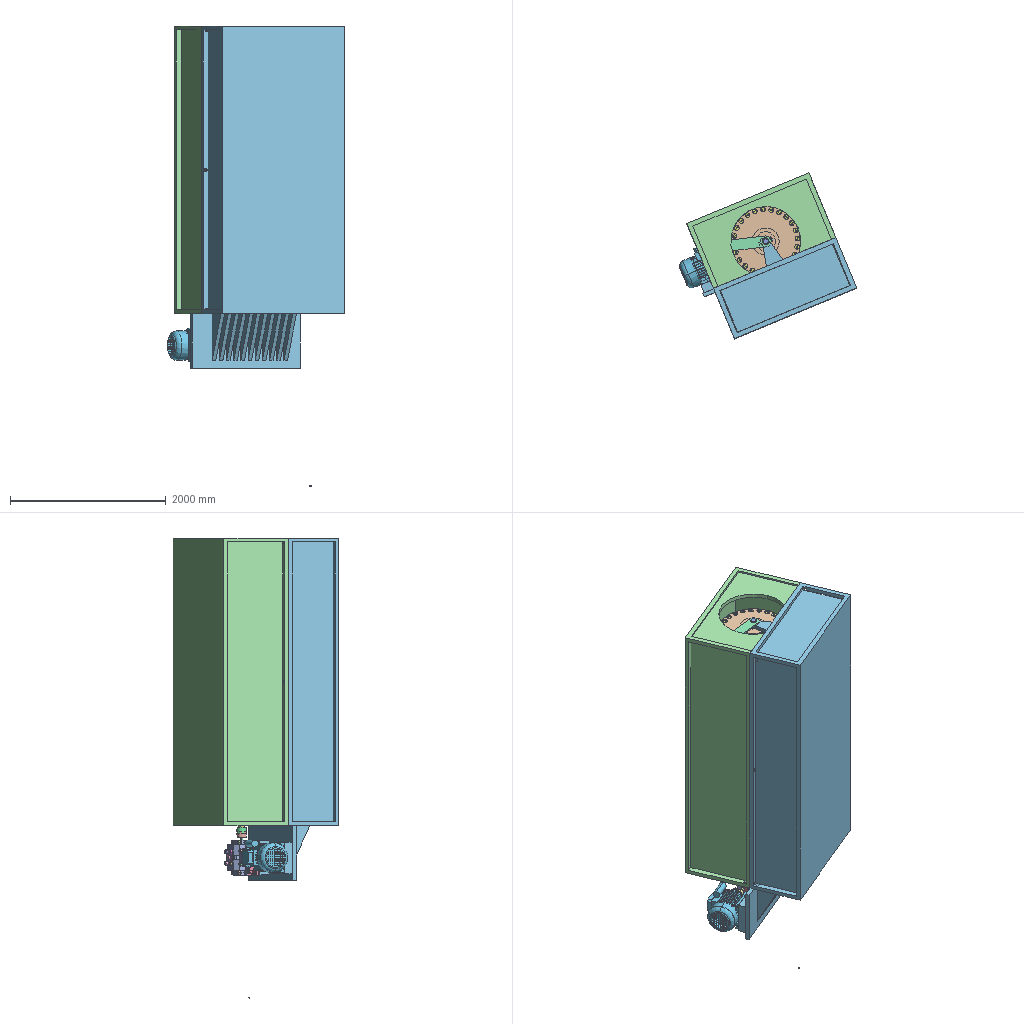Assembly | SolidWorks | 46 different items | 737 placed | box 2279 x 2129 x 5915 mm
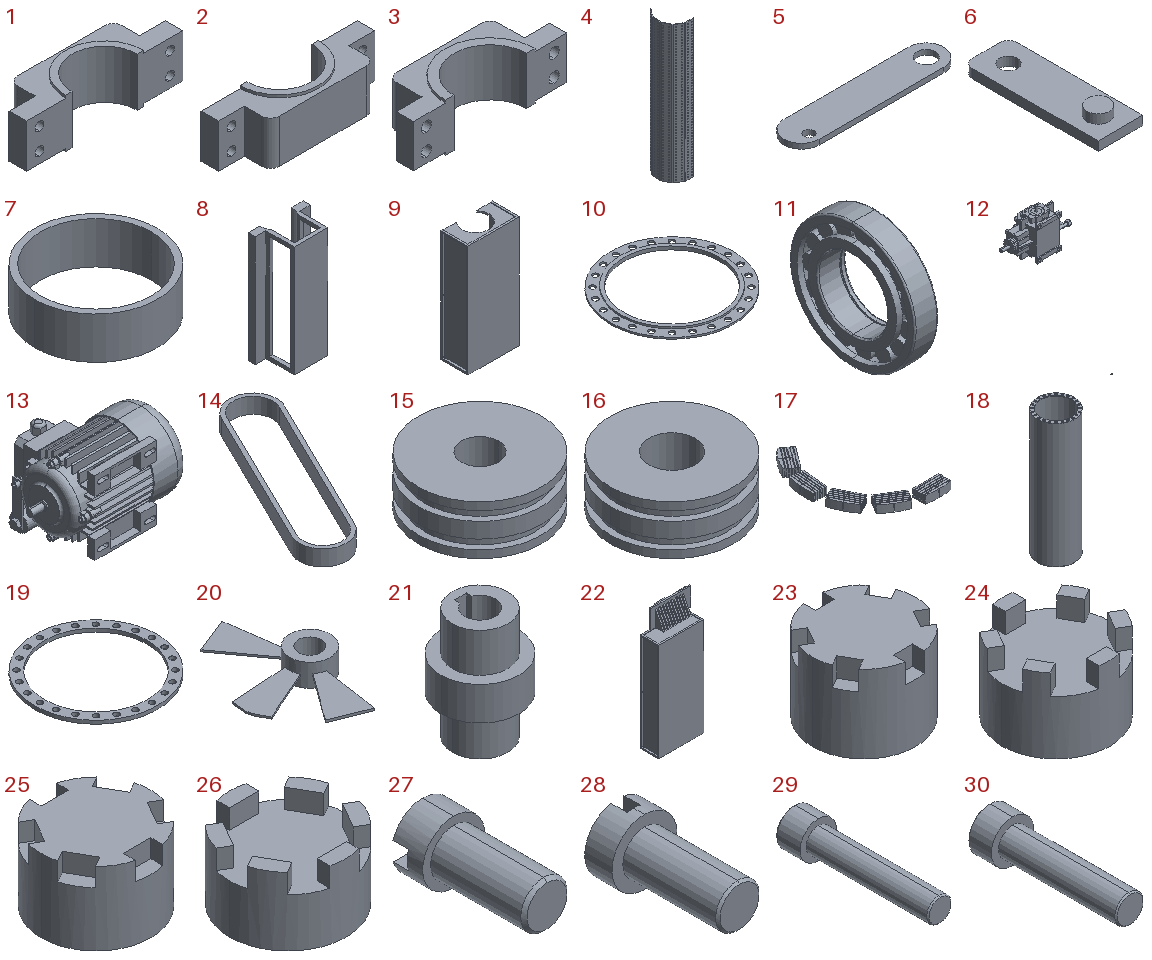Parts list (item | name | quantity | size | volume | features):
1 | - | x1 | 180 x 50 x 56 mm | 246956 mm3 | features ICE 4, Extrusion 1, Fillet 1, MirrorPattern 1
2 | - | x1 | 180 x 50 x 56 mm | 246956 mm3 | features ICE 4, Extrusion 1, Fillet 1, MirrorPattern 1
3 | - | x1 | 180 x 60 x 56 mm | 275897 mm3 | features ICE 4, Extrusion 1, Fillet 1, MirrorPattern 1
4 | - | x1 | 439.055 x 638.053 x 2960 mm | 32951018 mm3 | features ICE 7, 3DProfileFeature 3, Extrusion 1
5 | - | x1 | 640 x 140 x 20 mm | 1594386 mm3 | features Extrusion 1
6 | - | x1 | 100 x 300 x 40 mm | 610704 mm3 | features Extrusion 1, Fillet 1, ICE 1
7 | - | x1 | 100 x 100 x 34 mm | 50737 mm3 | features Extrusion 1
8 | - | x1 | 1550 x 1000 x 3127 mm | 797777759 mm3 | features ICE 10, Extrusion 1, MirrorPattern 1
9 | - | x1 | 1700 x 900 x 3700 mm | 580031915 mm3 | features ICE 37, Extrusion 1
10 | - | x1 | 900 x 900 x 25 mm | 3394255 mm3 | features ICE 3, Extrusion 1
11 | - | x2 | 40.8 x 180 x 180 mm | 440374 mm3 | features Revolution 4, CirPattern 1
12 | - | x1 | 1119 x 581.368 x 2095 mm | 29257315 mm3 | features BaseBody 37, Scale 1
13 | - | x1 | 643.342 x 464.31 x 414 mm | 44090407 mm3 | features ICE 21, Fillet 3, CirPattern 2, Revolution 2, LPattern 1, Scale 1
14 | - | x1 | 578.858 x 932.782 x 80 mm | 3573726 mm3 | features Extrusion 1
15 | - | x1 | 200 x 200 x 80 mm | 2108009 mm3 | features Extrusion 1, ICE 1, MirrorPattern 1
16 | - | x1 | 200 x 200 x 80 mm | 1980774 mm3 | features Extrusion 1, ICE 1, MirrorPattern 1
17 | - | x56 | 525 x 761.019 x 50 mm | 2587889 mm3 | features ICE 9, Extrusion 1
18 | - | x1 | 900 x 900 x 3000 mm | 71509466 mm3 | features ICE 2, Extrusion 1, MirrorPattern 1
19 | - | x1 | 900 x 900 x 25 mm | 4105669 mm3 | features ICE 2, Extrusion 1
20 | - | x17 | 431.967 x 677.234 x 100 mm | 2444150 mm3 | features ICE 4, Extrusion 1
21 | - | x1 | 70 x 70 x 100 mm | 224245 mm3 | features ICE 5, Extrusion 1
22 | - | x1 | 1850 x 1000 x 4400 mm | 1049313623 mm3 | features ICE 35, LPattern 2, Extrusion 1
23 | - | x1 | 80 x 80 x 60 mm | 237992 mm3 | features ICE 3, Extrusion 1
24 | - | x1 | 80 x 80 x 55 mm | 187551 mm3 | features ICE 3, Extrusion 1
25 | - | x1 | 120 x 120 x 80 mm | 586209 mm3 | features ICE 3, Extrusion 1
26 | - | x1 | 120 x 120 x 70 mm | 595667 mm3 | features ICE 3, Extrusion 1
27 | - | x560 | 20 x 40 x 20 mm | 7759 mm3 | features ICE 2, Chamfer 1, Extrusion 1
28 | - | x48 | 60 x 112.5 x 60 mm | 169671 mm3 | features ICE 2, Chamfer 1, Extrusion 1
29 | - | x4 | 15 x 60 x 15 mm | 5685 mm3 | features Chamfer 1, Extrusion 1, ICE 1
30 | - | x4 | 18 x 60 x 18 mm | 8188 mm3 | features Chamfer 1, Extrusion 1, ICE 1
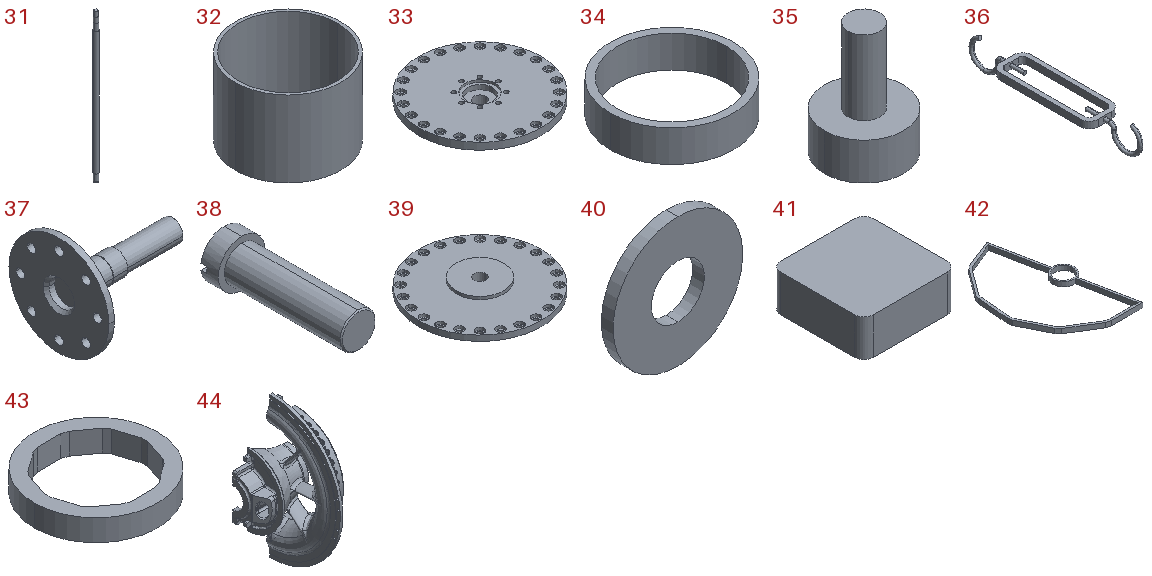31 | - | x1 | 100 x 100 x 3375 mm | 25329647 mm3 | features ICE 7, Chamfer 1, Extrusion 1
32 | - | x1 | 90 x 90 x 65 mm | 44670 mm3 | features Extrusion 1
33 | - | x1 | 900 x 900 x 130 mm | 35744082 mm3 | features ICE 6, CirPattern 2, Fillet 2, Extrusion 1, HoleWzd 1
34 | - | x1 | 85 x 85 x 22 mm | 27646 mm3 | features Extrusion 1
35 | - | x1 | 149.5 x 149.5 x 210 mm | 1568199 mm3 | features ICE 2, Extrusion 1
36 | - | x1 | 70 x 388 x 65.733 mm | 95929 mm3 | features Extrusion 1, ICE 1, MirrorPattern 1, Sweep 1
37 | - | x1 | 400 x 350 x 350 mm | 4309933 mm3 | features ICE 3, Chamfer 2, Revolution 1
38 | - | x8 | 40 x 115 x 40 mm | 88492 mm3 | features ICE 2, Chamfer 1, Extrusion 1
39 | - | x1 | 900 x 900 x 90 mm | 25700427 mm3 | features ICE 3, CirPattern 1, Extrusion 1, HoleWzd 1
40 | - | x1 | 220 x 20 x 220 mm | 633031 mm3 | features Extrusion 1
41 | - | x1 | 100 x 100 x 40 mm | 264030 mm3 | features Extrusion 1, Fillet 1, ICE 1
42 | - | x1 | 439.055 x 701.743 x 25 mm | 573866 mm3 | features ICE 2, Extrusion 1
43 | - | x1 | 884 x 884 x 155 mm | 38209027 mm3 | features Extrusion 1
44 | - | x1 | 985 x 1100 x 2200 mm | 275101534 mm3 | features MBimport 1
45 | UnnamedUnit | x1 | - | - | -
46 | Unnamed UnnamedGearUnnamedUnit (subassembly) | x1 | - | - | -
Mates (type | each side: item.copy, entity, surface, feature):
Concentric | 18.1 face cylinder Boss-Extrude 1 | 31.1 face cylinder Boss-Extrude 4
Concentric | 33.1 face cylinder Cut-Extrude 2 | 11.1 face cylinder Base-Revolve
Coincident | 11.1 face plane Boss-Revolve 2 | 40.1 face plane Boss-Extrude 1
Concentric | 18.1 face cylinder Cut-Extrude 1 | 33.1 face cylinder CirPattern 1
Concentric | 11.1 face cylinder Base-Revolve | 7.1 face cylinder Boss-Extrude 1
Coincident | 11.1 face plane Boss-Revolve 3 | 7.1 face plane Boss-Extrude 1
Concentric | 31.1 face cylinder Boss-Extrude 3 | 19.1 face cylinder Cut-Extrude 2
Concentric | 18.1 face cylinder Cut-Extrude 1 | 19.1 face cylinder Cut-Extrude 1
Coincident | 18.1 face plane Boss-Extrude 1 | 19.1 face plane Boss-Extrude 1
Coincident | 33.1 face plane Boss-Extrude 1 | 19.1 face plane Boss-Extrude 1
Concentric | 31.1 face cylinder Boss-Extrude 5 | 10.1 face cylinder Cut-Extrude 3
Concentric | 18.1 face cylinder Cut-Extrude 1 | 10.1 face cylinder Cut-Extrude 2
Coincident | 18.1 face plane Boss-Extrude 1 | 10.1 face plane Boss-Extrude 1
Concentric | 31.1 face cylinder Boss-Extrude 6 | 32.1 face cylinder Boss-Extrude 1
Concentric | 31.1 face cylinder Boss-Extrude 7 | 39.1 face cylinder Boss-Extrude 1
Concentric | 10.1 face cylinder Cut-Extrude 2 | 39.1 face cylinder CirPattern 1
Coincident | 10.1 face plane Boss-Extrude 1 | 39.1 face plane Boss-Extrude 1
Concentric | 31.1 face cylinder Boss-Extrude 7 | 34.1 face cylinder Boss-Extrude 1
Coincident | 39.1 face plane Boss-Extrude 3 | 34.1 edge
Coincident | 18.1 face plane Boss-Extrude 1 | 31.1 face plane Boss-Extrude 4
Concentric | 39.1 face cylinder Cut-Extrude 1 | 11.2 face cylinder Base-Revolve
Coincident | 39.1 face plane Boss-Extrude 1 | 11.2 face plane Boss-Revolve 2
Coincident | 31.1 face plane Boss-Extrude 5 | 32.1 face plane Boss-Extrude 1
Concentric | 31.1 face cylinder Boss-Extrude 7 | 2.1 face cylinder Cut-Extrude 1
Coincident | 39.1 face plane Boss-Extrude 3 | 2.1 face plane Mirror 1
Coincident | 10.1 face plane Boss-Extrude 2 | 4.1 face plane Boss-Extrude 1
Concentric | 18.1 face cylinder Boss-Extrude 1 | 17.1 face cylinder Boss-Extrude 1
Concentric | 39.1 face cylinder CirPattern 1 | 28.1 face cylinder Boss-Extrude 1
Coincident | 39.1 edge | 28.1 edge
Concentric | 33.1 face cylinder CirPattern 1 | 28.2 face cylinder Boss-Extrude 1
Coincident | 33.1 edge | 28.2 face plane Boss-Extrude 2
Concentric | 31.1 face cylinder Boss-Extrude 4 | 20.1 face cylinder Boss-Extrude 3
DistanceDim | 20.1 face plane Boss-Extrude 2 | 33.1 face plane Boss-Extrude 1
Coincident | 22.1 face plane | 5.1 face plane Boss-Extrude 1
Concentric | 22.1 edge | 6.1 edge
Coincident | 22.1 face plane | 6.1 face plane Boss-Extrude 2
Parallel | 36.1 edge | assembly select_type:10
Parallel | 3.1 edge | 22.1 face plane
Concentric | 2.1 face cylinder Cut-Extrude 2 | 29.1 face cylinder Boss-Extrude 1
Coincident | 2.1 face plane Boss-Extrude 3 | 29.1 face plane Boss-Extrude 2
Concentric | 2.1 face cylinder Cut-Extrude 2 | 29.2 face cylinder Boss-Extrude 1
Coincident | 2.1 face plane Boss-Extrude 3 | 29.2 face plane Boss-Extrude 2
Concentric | 2.1 face cylinder Cut-Extrude 2 | 29.3 face cylinder Boss-Extrude 1
Coincident | 2.1 face plane Boss-Extrude 3 | 29.3 edge
Concentric | 2.1 face cylinder Cut-Extrude 2 | 29.4 face cylinder Boss-Extrude 1
Coincident | 2.1 face plane Boss-Extrude 3 | 29.4 face plane Boss-Extrude 2
Concentric | 3.1 face cylinder Cut-Extrude 2 | 30.1 face cylinder Boss-Extrude 1
Coincident | 3.1 face plane Boss-Extrude 2 | 30.1 face plane Boss-Extrude 2
Concentric | 3.1 face cylinder Cut-Extrude 2 | 30.2 face cylinder Boss-Extrude 1
Coincident | 3.1 face plane Boss-Extrude 2 | 30.2 face plane Boss-Extrude 2
Concentric | 3.1 face cylinder Cut-Extrude 2 | 30.3 face cylinder Boss-Extrude 1
Coincident | 3.1 face plane Boss-Extrude 2 | 30.3 edge
Concentric | 3.1 edge | 30.4 face cylinder Boss-Extrude 1
Coincident | 3.1 face plane Boss-Extrude 2 | 30.4 face plane Boss-Extrude 2
Concentric | 17.1 face cylinder Cut-Extrude 9 | 4.1 face cylinder Cut-Extrude 5
Concentric | 4.1 edge | 27.1 face cylinder Boss-Extrude 1
Coincident | 4.1 face plane Boss-Extrude 1 | 27.1 edge
Concentric | 4.1 face cylinder Cut-Extrude 5 | 27.2 face cylinder Boss-Extrude 1
Coincident | 4.1 face plane Boss-Extrude 1 | 27.2 edge
Concentric | 4.1 face cylinder Cut-Extrude 6 | 27.3 face cylinder Boss-Extrude 1
Coincident | 4.1 face plane Boss-Extrude 1 | 27.3 face plane Boss-Extrude 2
Concentric | 4.1 face cylinder Cut-Extrude 6 | 27.4 face cylinder Boss-Extrude 1
Coincident | 4.1 face plane Boss-Extrude 1 | 27.4 edge
Concentric | 4.1 face cylinder Cut-Extrude 3 | 27.5 face cylinder Boss-Extrude 1
Coincident | 4.1 face plane Boss-Extrude 1 | 27.5 edge
Concentric | 4.1 edge | 27.6 face cylinder Boss-Extrude 1
Coincident | 4.1 face plane Boss-Extrude 1 | 27.6 face plane Boss-Extrude 2
Concentric | 4.1 edge | 27.7 face cylinder Boss-Extrude 1
Coincident | 4.1 face plane Boss-Extrude 1 | 27.7 edge
Concentric | 4.1 face cylinder Cut-Extrude 2 | 27.8 face cylinder Boss-Extrude 1
Coincident | 4.1 face plane Boss-Extrude 1 | 27.8 edge
Concentric | 4.1 edge | 27.9 face cylinder Boss-Extrude 1
Coincident | 4.1 face plane Boss-Extrude 1 | 27.9 edge
Concentric | 4.1 face cylinder Cut-Extrude 1 | 27.10 face cylinder Boss-Extrude 1
Coincident | 4.1 face plane Boss-Extrude 1 | 27.10 face plane Boss-Extrude 2
Coincident | 4.1 edge | 20.1 face plane Boss-Extrude 1
Coincident | 4.1 edge | 17.2 face plane Cut-Extrude 2
Parallel | 27.1 edge | 4.1 edge
Concentric | 31.1 face cylinder Boss-Extrude 3 | 22.1 face cylinder
Concentric | 22.1 edge | 29.3 face cylinder Boss-Extrude 1
Concentric | 22.1 face cylinder | 30.1 face cylinder Boss-Extrude 1
Coincident | 3.1 face plane Boss-Extrude 1 | 22.1 face plane
Concentric | 33.1 edge | 37.1 face cylinder Cut-Extrude 3
Concentric | 37.1 face cylinder Cut-Extrude 3 | 38.1 face cylinder Boss-Extrude 1
Concentric | 31.1 face cylinder Boss-Extrude 3 | 40.1 face cylinder Boss-Extrude 1
Coincident | 33.1 face plane Boss-Extrude 1 | 40.1 face plane Boss-Extrude 1
Concentric | 31.1 face cylinder Boss-Extrude 3 | 37.1 face cylinder Cut-Extrude 1
Coincident | 37.1 face plane Revolve 1 | 38.1 edge
Coincident | 33.1 face plane Boss-Extrude 1 | 37.1 face plane Revolve 1
Concentric | 22.1 face cylinder | 9.1 face cylinder Cut-Extrude 20
Concentric | 22.1 edge | 9.1 face cylinder Cut-Extrude 20
Parallel | 22.1 edge | 12.1 edge | 2 times
Parallel | 22.1 edge | 13.1 edge | 2 times
Concentric | 12.1 face cylinder UnnamedGear 17Unnamed InputShaft-1-solid1 | 13.1 face cylinder Revolve 1
Concentric | 37.1 face cylinder Revolve 1 | 12.1 face cylinder UnnamedGear 34Unnamed OutputShaft-1-solid1
Parallel | 22.1 face plane | 13.1 face plane Boss-Extrude 9
Coincident | 22.1 face plane | 9.1 face plane Boss-Extrude 9
Coincident | 12.1 face plane UnnamedGear 17Unnamed InputShaft-1-solid1 | 23.1 face plane Cut-Extrude 1
Concentric | 12.1 face cylinder UnnamedGear 17Unnamed InputShaft-1-solid1 | 23.1 face cylinder Boss-Extrude 1
Concentric | 13.1 face cylinder Revolve 1 | 24.1 edge
Coincident | 13.1 edge | 24.1 edge
Coincident | 23.1 face plane Boss-Extrude 1 | 24.1 face plane Boss-Extrude 1
Coincident | 23.1 face plane Cut-Extrude 2 | 24.1 face plane Boss-Extrude 2
Concentric | 37.1 face cylinder Revolve 1 | 25.1 face cylinder Cut-Extrude 1
Coincident | 37.1 face plane Revolve 1 | 25.1 edge
Concentric | 12.1 face cylinder UnnamedGear 34Unnamed OutputShaft-1-solid1 | 26.1 face cylinder Cut-Extrude 1
Coincident | 12.1 edge | 26.1 face plane Cut-Extrude 1
Coincident | 25.1 face plane Boss-Extrude 1 | 26.1 face plane Boss-Extrude 1
Coincident | 25.1 face plane Cut-Extrude 2 | 26.1 face plane Boss-Extrude 2